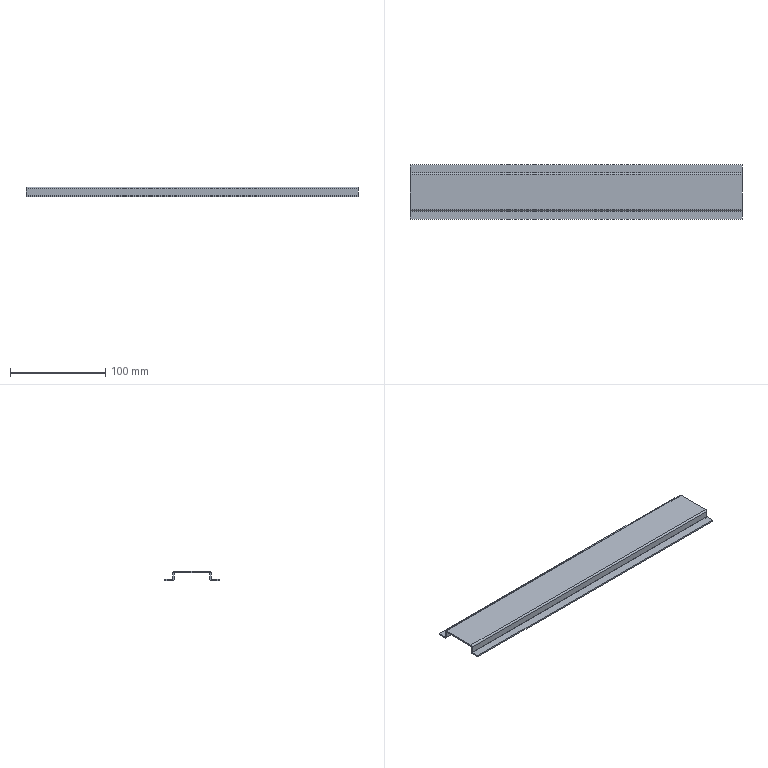Part | STEP file | FHD-021-004-C rear door reinforcing rib | 1 solid | 22 faces | box 348 x 57 x 10 mm | volume 37777 mm3 | plane 14 | cylinder 8 | commonest cylinder face diameters 0.4 x4 3.4 x4